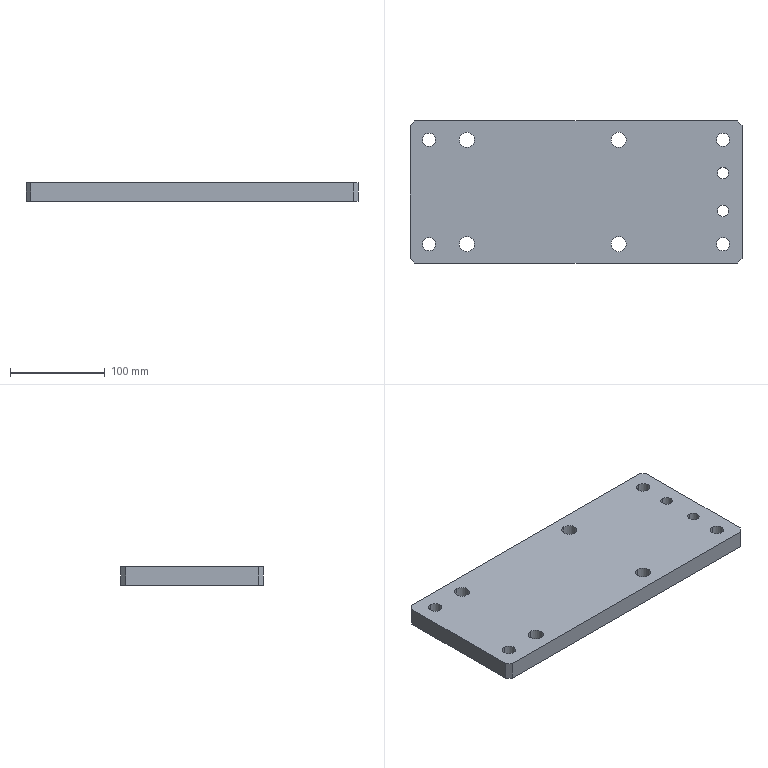Part | STEP file | J451-EBZ05-07-00-Part-1 | 1 solid | 30 faces | box 350 x 150 x 19 mm | volume 965272 mm3 | cylinder 20 | plane 10 | commonest cylinder face diameters 14 x8 16 x8 12 x4